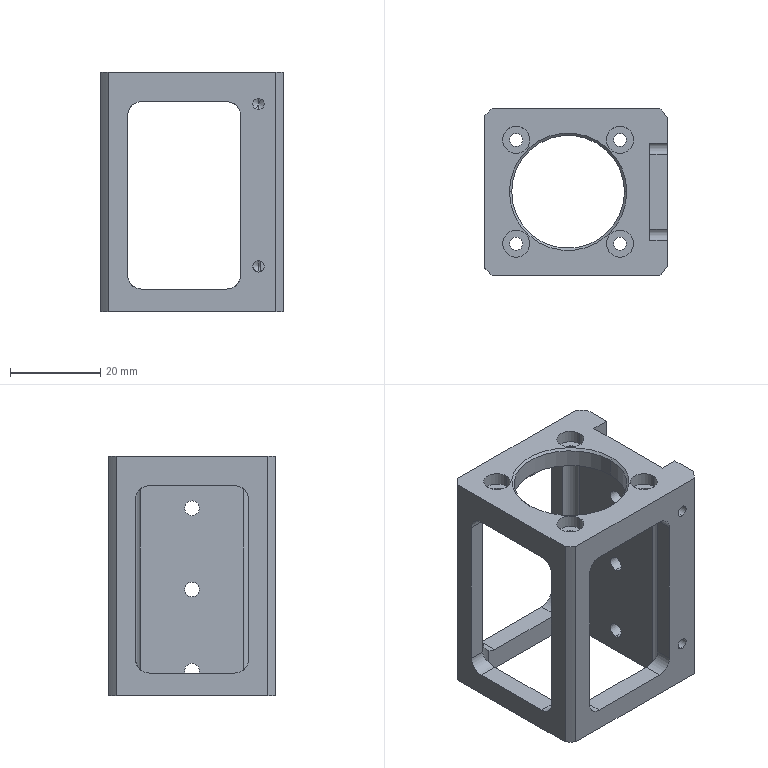Part | STEP file | 1 solid | 153 faces | box 40.5 x 37 x 53 mm | volume 18902 mm3 | cylinder 81 | plane 54 | cone 18 | commonest cylinder face diameters 6 x20 8 x16 2.05 x12 2.9 x8 3.3 x6 4 x6